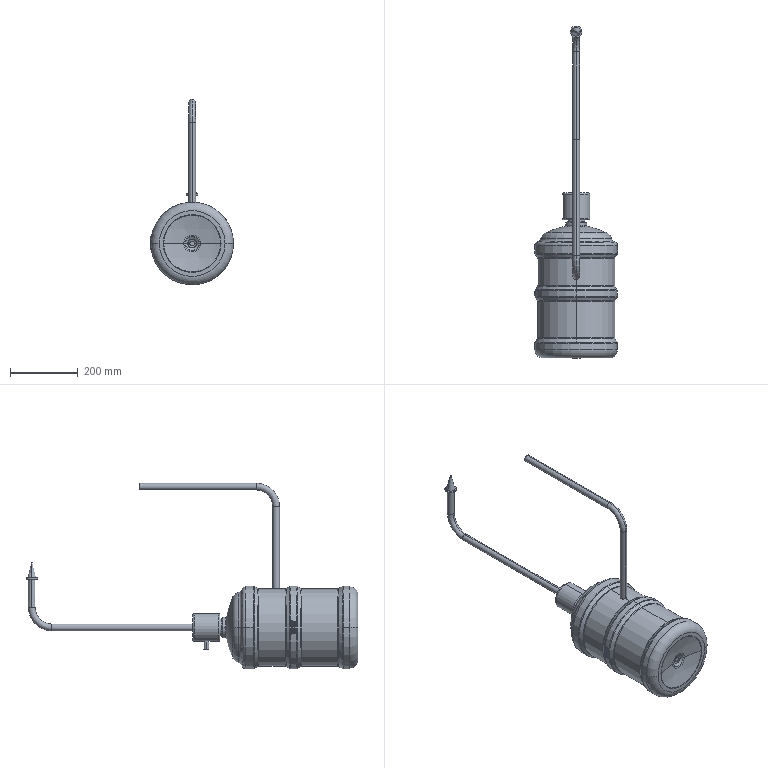Part | SolidWorks | features Split 3, Revolution 2, Sweep 2, BaseBody 1, DelFace 1, Fillet 1, ICE 1 | 5 solids | 614 faces | box 245.999 x 983.22 x 550.042 mm | volume 1897032 mm3 | spline 399 | torus 82 | cylinder 71 | plane 32 | cone 26 | sphere 4 | commonest cylinder face diameters 20 x12 245 x11 247 x11 230 x6 239 x6 2 x4